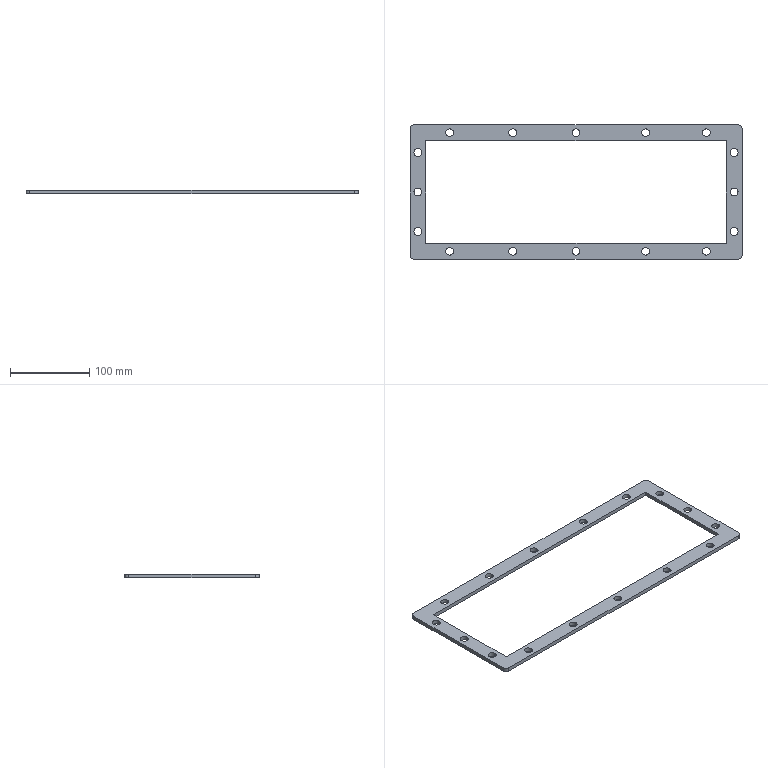Part | NX | features BREP 1 | 1 solid | 46 faces | box 420 x 170 x 5 mm | volume 103610 mm3 | cylinder 36 | plane 10 | commonest cylinder face diameters 10 x36